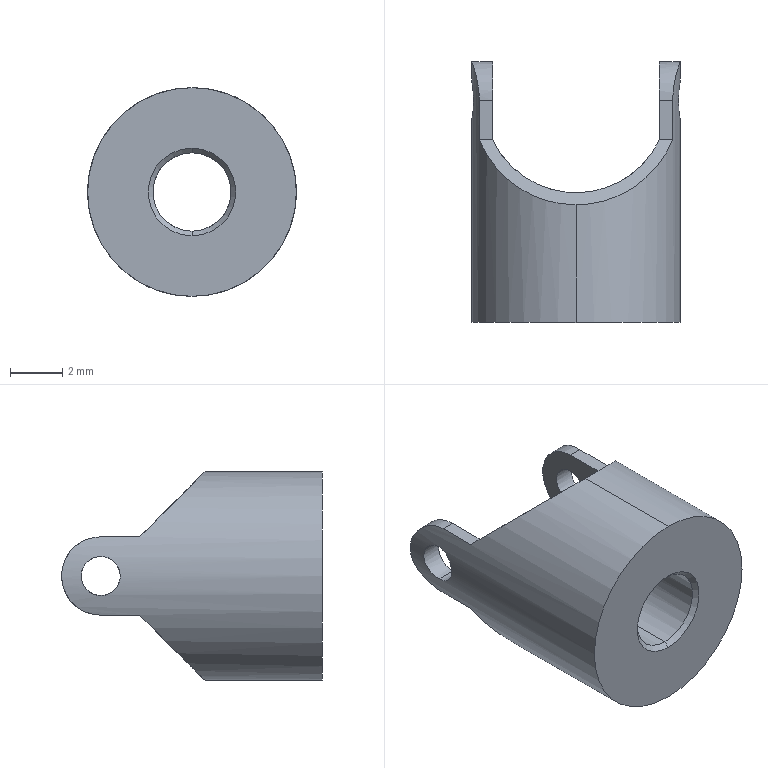Part | SolidWorks | features BaseBody 1, Scale 1 | 1 solid | 22 faces | box 8 x 10 x 8 mm | volume 253.333 mm3 | cylinder 11 | plane 9 | cone 2 | commonest cylinder face diameters 1.5 x4 3 x4 8 x2 7.068 x1
STEP:
#1=CARTESIAN_POINT('',(-3.2,8.5,-0.75));
#2=VERTEX_POINT('',#1);
#3=CARTESIAN_POINT('',(-3.2,8.5,0.75));
#4=VERTEX_POINT('',#3);
#5=CARTESIAN_POINT('',(-3.2,8.5,0.));
#6=DIRECTION('',(-1.,0.,0.));
#7=DIRECTION('',(0.,0.,-1.));
#8=AXIS2_PLACEMENT_3D('',#5,#6,#7);
#9=CIRCLE('',#8,0.75);
#10=EDGE_CURVE('',#2,#4,#9,.T.);
#11=ORIENTED_EDGE('',*,*,#10,.F.);
#12=CARTESIAN_POINT('',(-3.929,8.5,-0.75));
#13=VERTEX_POINT('',#12);
#14=CARTESIAN_POINT('',(4.,8.5,-0.75));
#15=DIRECTION('',(-1.,0.,0.));
#16=VECTOR('',#15,1000.);
#17=LINE('',#14,#16);
#18=EDGE_CURVE('',#2,#13,#17,.T.);
#19=ORIENTED_EDGE('',*,*,#18,.T.);
#20=CARTESIAN_POINT('',(-3.929,8.5,0.75));
#21=VERTEX_POINT('',#20);
#22=CARTESIAN_POINT('',(-3.929,8.5,0.75));
#23=CARTESIAN_POINT('',(-3.929,8.301,0.75));
#24=CARTESIAN_POINT('',(-3.946,8.107,0.668));
#25=CARTESIAN_POINT('',(-3.974,7.9,0.461));
#26=CARTESIAN_POINT('',(-3.983,7.845,0.3777));
#27=CARTESIAN_POINT('',(-3.996,7.77,0.1965));
#28=CARTESIAN_POINT('',(-4.,7.75,0.09865));
#29=CARTESIAN_POINT('',(-4.,7.75,-0.1985));
#30=CARTESIAN_POINT('',(-3.983,7.832,-0.3925));
#31=CARTESIAN_POINT('',(-3.946,8.108,-0.6688));
#32=CARTESIAN_POINT('',(-3.929,8.304,-0.75));
#33=CARTESIAN_POINT('',(-3.929,8.5,-0.75));
#34=B_SPLINE_CURVE_WITH_KNOTS('',3,(#22,#23,#24,#25,#26,#27,#28,#29,#30,#31,#32,#33),.UNSPECIFIED.,.F.,.F.,(4,2,2,2,2,4),(0.,0.0005912,0.0008868,0.001182,0.001774,0.002365),.UNSPECIFIED.);
#35=EDGE_CURVE('',#21,#13,#34,.T.);
#36=ORIENTED_EDGE('',*,*,#35,.F.);
#37=CARTESIAN_POINT('',(4.,8.5,0.75));
#38=DIRECTION('',(-1.,0.,0.));
#39=VECTOR('',#38,1000.);
#40=LINE('',#37,#39);
#41=EDGE_CURVE('',#4,#21,#40,.T.);
#42=ORIENTED_EDGE('',*,*,#41,.F.);
#43=EDGE_LOOP('',(#11,#19,#36,#42));
#44=FACE_OUTER_BOUND('',#43,.T.);
#45=CARTESIAN_POINT('',(4.,8.5,0.));
#46=DIRECTION('',(-1.,0.,0.));
#47=DIRECTION('',(0.,0.,1.));
#48=AXIS2_PLACEMENT_3D('',#45,#46,#47);
#49=CYLINDRICAL_SURFACE('',#48,0.75);
#50=ADVANCED_FACE('',(#44),#49,.F.);
#51=CARTESIAN_POINT('',(3.929,8.5,-0.75));
#52=VERTEX_POINT('',#51);
#53=CARTESIAN_POINT('',(3.929,8.5,0.75));
#54=VERTEX_POINT('',#53);
#55=CARTESIAN_POINT('',(3.929,8.5,-0.75));
#56=CARTESIAN_POINT('',(3.929,8.402,-0.75));
#57=CARTESIAN_POINT('',(3.933,8.303,-0.7304));
#58=CARTESIAN_POINT('',(3.946,8.122,-0.6552));
#59=CARTESIAN_POINT('',(3.955,8.039,-0.6001));
#60=CARTESIAN_POINT('',(3.974,7.9,-0.4606));
#61=CARTESIAN_POINT('',(3.983,7.845,-0.3781));
#62=CARTESIAN_POINT('',(3.996,7.769,-0.1962));
#63=CARTESIAN_POINT('',(4.,7.75,-0.09779));
#64=CARTESIAN_POINT('',(4.,7.75,0.1964));
#65=CARTESIAN_POINT('',(3.983,7.832,0.3921));
#66=CARTESIAN_POINT('',(3.955,8.039,0.5993));
#67=CARTESIAN_POINT('',(3.946,8.122,0.655));
#68=CARTESIAN_POINT('',(3.933,8.303,0.7304));
#69=CARTESIAN_POINT('',(3.929,8.401,0.75));
#70=CARTESIAN_POINT('',(3.929,8.5,0.75));
#71=B_SPLINE_CURVE_WITH_KNOTS('',3,(#55,#56,#57,#58,#59,#60,#61,#62,#63,#64,#65,#66,#67,#68,#69,#70),.UNSPECIFIED.,.F.,.F.,(4,2,2,2,2,2,2,4),(0.002365,0.00266,0.002956,0.003252,0.003547,0.004139,0.004434,0.00473),.UNSPECIFIED.);
#72=EDGE_CURVE('',#52,#54,#71,.T.);
#73=ORIENTED_EDGE('',*,*,#72,.F.);
#74=CARTESIAN_POINT('',(3.2,8.5,-0.75));
#75=VERTEX_POINT('',#74);
#76=CARTESIAN_POINT('',(4.,8.5,-0.75));
#77=DIRECTION('',(-1.,0.,0.));
#78=VECTOR('',#77,1000.);
#79=LINE('',#76,#78);
#80=EDGE_CURVE('',#52,#75,#79,.T.);
#81=ORIENTED_EDGE('',*,*,#80,.T.);
#82=CARTESIAN_POINT('',(3.2,8.5,0.75));
#83=VERTEX_POINT('',#82);
#84=CARTESIAN_POINT('',(3.2,8.5,0.));
#85=DIRECTION('',(1.,0.,0.));
#86=DIRECTION('',(0.,0.,1.));
#87=AXIS2_PLACEMENT_3D('',#84,#85,#86);
#88=CIRCLE('',#87,0.75);
#89=EDGE_CURVE('',#83,#75,#88,.T.);
#90=ORIENTED_EDGE('',*,*,#89,.F.);
#91=CARTESIAN_POINT('',(4.,8.5,0.75));
#92=DIRECTION('',(-1.,0.,0.));
#93=VECTOR('',#92,1000.);
#94=LINE('',#91,#93);
#95=EDGE_CURVE('',#54,#83,#94,.T.);
#96=ORIENTED_EDGE('',*,*,#95,.F.);
#97=EDGE_LOOP('',(#73,#81,#90,#96));
#98=FACE_OUTER_BOUND('',#97,.T.);
#99=CARTESIAN_POINT('',(4.,8.5,0.));
#100=DIRECTION('',(-1.,0.,0.));
#101=DIRECTION('',(0.,0.,1.));
#102=AXIS2_PLACEMENT_3D('',#99,#100,#101);
#103=CYLINDRICAL_SURFACE('',#102,0.75);
#104=ADVANCED_FACE('',(#98),#103,.F.);
#105=CARTESIAN_POINT('',(3.929,8.5,0.75));
#106=CARTESIAN_POINT('',(3.929,8.699,0.75));
#107=CARTESIAN_POINT('',(3.946,8.893,0.668));
#108=CARTESIAN_POINT('',(3.974,9.1,0.461));
#109=CARTESIAN_POINT('',(3.983,9.155,0.3777));
#110=CARTESIAN_POINT('',(3.996,9.23,0.1965));
#111=CARTESIAN_POINT('',(4.,9.25,0.09865));
#112=CARTESIAN_POINT('',(4.,9.25,-0.1985));
#113=CARTESIAN_POINT('',(3.983,9.168,-0.3925));
#114=CARTESIAN_POINT('',(3.946,8.892,-0.6688));
#115=CARTESIAN_POINT('',(3.929,8.696,-0.75));
#116=CARTESIAN_POINT('',(3.929,8.5,-0.75));
#117=B_SPLINE_CURVE_WITH_KNOTS('',3,(#105,#106,#107,#108,#109,#110,#111,#112,#113,#114,#115,#116),.UNSPECIFIED.,.F.,.F.,(4,2,2,2,2,4),(0.,0.0005912,0.0008868,0.001182,0.001774,0.002365),.UNSPECIFIED.);
#118=EDGE_CURVE('',#54,#52,#117,.T.);
#119=ORIENTED_EDGE('',*,*,#118,.T.);
#120=ORIENTED_EDGE('',*,*,#72,.T.);
#121=EDGE_LOOP('',(#119,#120));
#122=FACE_BOUND('',#121,.T.);
#123=CARTESIAN_POINT('',(0.,4.5,4.));
#124=VERTEX_POINT('',#123);
#125=CARTESIAN_POINT('',(3.708,7.,1.5));
#126=VERTEX_POINT('',#125);
#127=CARTESIAN_POINT('',(0.,4.5,4.));
#128=CARTESIAN_POINT('',(1.682,4.5,4.));
#129=CARTESIAN_POINT('',(3.077,5.44,3.06));
#130=CARTESIAN_POINT('',(3.708,7.,1.5));
#131=(BOUNDED_CURVE()B_SPLINE_CURVE(3,(#127,#128,#129,#130),.UNSPECIFIED.,.F.,.F.)B_SPLINE_CURVE_WITH_KNOTS((4,4),(0.,1.186),.UNSPECIFIED.)CURVE()GEOMETRIC_REPRESENTATION_ITEM()RATIONAL_B_SPLINE_CURVE((1.,0.8861,0.8861,1.))REPRESENTATION_ITEM(''));
#132=EDGE_CURVE('',#124,#126,#131,.T.);
#133=ORIENTED_EDGE('',*,*,#132,.F.);
#134=CARTESIAN_POINT('',(0.,0.,4.));
#135=VERTEX_POINT('',#134);
#136=CARTESIAN_POINT('',(0.,10.,4.));
#137=DIRECTION('',(0.,-1.,0.));
#138=VECTOR('',#137,1000.);
#139=LINE('',#136,#138);
#140=EDGE_CURVE('',#124,#135,#139,.T.);
#141=ORIENTED_EDGE('',*,*,#140,.T.);
#142=CARTESIAN_POINT('',(0.,0.,-4.));
#143=VERTEX_POINT('',#142);
#144=CARTESIAN_POINT('',(0.,0.,0.));
#145=DIRECTION('',(0.,1.,0.));
#146=DIRECTION('',(1.,0.,0.));
#147=AXIS2_PLACEMENT_3D('',#144,#145,#146);
#148=CIRCLE('',#147,4.);
#149=EDGE_CURVE('',#135,#143,#148,.T.);
#150=ORIENTED_EDGE('',*,*,#149,.T.);
#151=CARTESIAN_POINT('',(0.,4.5,-4.));
#152=VERTEX_POINT('',#151);
#153=CARTESIAN_POINT('',(0.,10.,-4.));
#154=DIRECTION('',(0.,-1.,0.));
#155=VECTOR('',#154,1000.);
#156=LINE('',#153,#155);
#157=EDGE_CURVE('',#152,#143,#156,.T.);
#158=ORIENTED_EDGE('',*,*,#157,.F.);
#159=CARTESIAN_POINT('',(3.708,7.,-1.5));
#160=VERTEX_POINT('',#159);
#161=CARTESIAN_POINT('',(3.708,7.,-1.5));
#162=CARTESIAN_POINT('',(3.077,5.44,-3.06));
#163=CARTESIAN_POINT('',(1.682,4.5,-4.));
#164=CARTESIAN_POINT('',(0.,4.5,-4.));
#165=(BOUNDED_CURVE()B_SPLINE_CURVE(3,(#161,#162,#163,#164),.UNSPECIFIED.,.F.,.F.)B_SPLINE_CURVE_WITH_KNOTS((4,4),(5.097,6.283),.UNSPECIFIED.)CURVE()GEOMETRIC_REPRESENTATION_ITEM()RATIONAL_B_SPLINE_CURVE((1.,0.8861,0.8861,1.))REPRESENTATION_ITEM(''));
#166=EDGE_CURVE('',#160,#152,#165,.T.);
#167=ORIENTED_EDGE('',*,*,#166,.F.);
#168=CARTESIAN_POINT('',(3.708,8.5,-1.5));
#169=VERTEX_POINT('',#168);
#170=CARTESIAN_POINT('',(3.708,10.,-1.5));
#171=DIRECTION('',(0.,-1.,0.));
#172=VECTOR('',#171,1000.);
#173=LINE('',#170,#172);
#174=EDGE_CURVE('',#169,#160,#173,.T.);
#175=ORIENTED_EDGE('',*,*,#174,.F.);
#176=CARTESIAN_POINT('',(3.708,8.5,1.5));
#177=VERTEX_POINT('',#176);
#178=CARTESIAN_POINT('',(3.708,8.5,1.5));
#179=CARTESIAN_POINT('',(3.708,8.6,1.5));
#180=CARTESIAN_POINT('',(3.712,8.698,1.49));
#181=CARTESIAN_POINT('',(3.727,8.891,1.451));
#182=CARTESIAN_POINT('',(3.739,8.987,1.422));
#183=CARTESIAN_POINT('',(3.781,9.258,1.309));
#184=CARTESIAN_POINT('',(3.819,9.423,1.198));
#185=CARTESIAN_POINT('',(3.894,9.697,0.924));
#186=CARTESIAN_POINT('',(3.932,9.809,0.7582));
#187=CARTESIAN_POINT('',(3.971,9.922,0.488));
#188=CARTESIAN_POINT('',(3.982,9.951,0.3926));
#189=CARTESIAN_POINT('',(3.996,9.99,0.1986));
#190=CARTESIAN_POINT('',(4.,10.,0.1006));
#191=CARTESIAN_POINT('',(4.,10.,-0.09712));
#192=CARTESIAN_POINT('',(3.996,9.99,-0.1975));
#193=CARTESIAN_POINT('',(3.982,9.952,-0.3907));
#194=CARTESIAN_POINT('',(3.972,9.923,-0.4847));
#195=CARTESIAN_POINT('',(3.932,9.809,-0.759));
#196=CARTESIAN_POINT('',(3.895,9.698,-0.9229));
#197=CARTESIAN_POINT('',(3.838,9.492,-1.129));
#198=CARTESIAN_POINT('',(3.819,9.417,-1.191));
#199=CARTESIAN_POINT('',(3.783,9.256,-1.299));
#200=CARTESIAN_POINT('',(3.767,9.168,-1.347));
#201=CARTESIAN_POINT('',(3.725,8.898,-1.459));
#202=CARTESIAN_POINT('',(3.708,8.7,-1.5));
#203=CARTESIAN_POINT('',(3.708,8.5,-1.5));
#204=B_SPLINE_CURVE_WITH_KNOTS('',3,(#178,#179,#180,#181,#182,#183,#184,#185,#186,#187,#188,#189,#190,#191,#192,#193,#194,#195,#196,#197,#198,#199,#200,#201,#202,#203),.UNSPECIFIED.,.F.,.F.,(4,2,2,2,2,2,2,2,2,2,2,2,4),(0.,0.0002957,0.0005914,0.001183,0.001774,0.00207,0.002366,0.002661,0.002957,0.003548,0.003844,0.00414,0.004731),.UNSPECIFIED.);
#205=EDGE_CURVE('',#177,#169,#204,.T.);
#206=ORIENTED_EDGE('',*,*,#205,.F.);
#207=CARTESIAN_POINT('',(3.708,10.,1.5));
#208=DIRECTION('',(0.,1.,0.));
#209=VECTOR('',#208,1000.);
#210=LINE('',#207,#209);
#211=EDGE_CURVE('',#126,#177,#210,.T.);
#212=ORIENTED_EDGE('',*,*,#211,.F.);
#213=EDGE_LOOP('',(#133,#141,#150,#158,#167,#175,#206,#212));
#214=FACE_OUTER_BOUND('',#213,.T.);
#215=CARTESIAN_POINT('',(0.,10.,0.));
#216=DIRECTION('',(0.,-1.,0.));
#217=DIRECTION('',(0.,0.,-1.));
#218=AXIS2_PLACEMENT_3D('',#215,#216,#217);
#219=CYLINDRICAL_SURFACE('',#218,4.);
#220=ADVANCED_FACE('',(#122,#214),#219,.T.);
#221=CARTESIAN_POINT('',(0.,4.966,1.5));
#222=VERTEX_POINT('',#221);
#223=CARTESIAN_POINT('',(0.,4.966,-1.5));
#224=VERTEX_POINT('',#223);
#225=CARTESIAN_POINT('',(0.,4.966,1.5));
#226=CARTESIAN_POINT('',(-0.09881,4.966,1.5));
#227=CARTESIAN_POINT('',(-0.1992,4.97,1.49));
#228=CARTESIAN_POINT('',(-0.3935,4.987,1.451));
#229=CARTESIAN_POINT('',(-0.4874,4.998,1.422));
#230=CARTESIAN_POINT('',(-0.76,5.044,1.308));
#231=CARTESIAN_POINT('',(-0.9239,5.086,1.198));
#232=CARTESIAN_POINT('',(-1.13,5.151,0.9907));
#233=CARTESIAN_POINT('',(-1.192,5.172,0.916));
#234=CARTESIAN_POINT('',(-1.3,5.213,0.7551));
#235=CARTESIAN_POINT('',(-1.347,5.232,0.6678));
#236=CARTESIAN_POINT('',(-1.422,5.264,0.4871));
#237=CARTESIAN_POINT('',(-1.451,5.277,0.3937));
#238=CARTESIAN_POINT('',(-1.49,5.295,0.2));
#239=CARTESIAN_POINT('',(-1.5,5.3,0.09937));
#240=CARTESIAN_POINT('',(-1.5,5.3,-0.1973));
#241=CARTESIAN_POINT('',(-1.46,5.28,-0.3966));
#242=CARTESIAN_POINT('',(-1.347,5.232,-0.6676));
#243=CARTESIAN_POINT('',(-1.3,5.213,-0.755));
#244=CARTESIAN_POINT('',(-1.192,5.172,-0.9164));
#245=CARTESIAN_POINT('',(-1.13,5.151,-0.9911));
#246=CARTESIAN_POINT('',(-0.9236,5.086,-1.198));
#247=CARTESIAN_POINT('',(-0.7612,5.044,-1.308));
#248=CARTESIAN_POINT('',(-0.3959,4.983,-1.46));
#249=CARTESIAN_POINT('',(-0.2006,4.966,-1.5));
#250=CARTESIAN_POINT('',(0.,4.966,-1.5));
#251=B_SPLINE_CURVE_WITH_KNOTS('',3,(#225,#226,#227,#228,#229,#230,#231,#232,#233,#234,#235,#236,#237,#238,#239,#240,#241,#242,#243,#244,#245,#246,#247,#248,#249,#250),.UNSPECIFIED.,.F.,.F.,(4,2,2,2,2,2,2,2,2,2,2,2,4),(0.004747,0.005043,0.005339,0.005932,0.006229,0.006525,0.006822,0.007118,0.007711,0.008007,0.008304,0.008896,0.009489),.UNSPECIFIED.);
#252=EDGE_CURVE('',#222,#224,#251,.T.);
#253=ORIENTED_EDGE('',*,*,#252,.F.);
#254=CARTESIAN_POINT('',(0.,0.18,1.5));
#255=VERTEX_POINT('',#254);
#256=CARTESIAN_POINT('',(0.,15.1,1.5));
#257=DIRECTION('',(0.,-1.,0.));
#258=VECTOR('',#257,1000.);
#259=LINE('',#256,#258);
#260=EDGE_CURVE('',#222,#255,#259,.T.);
#261=ORIENTED_EDGE('',*,*,#260,.T.);
#262=CARTESIAN_POINT('',(0.,0.18,-1.5));
#263=VERTEX_POINT('',#262);
#264=CARTESIAN_POINT('',(0.,0.18,0.));
#265=DIRECTION('',(0.,-1.,0.));
#266=DIRECTION('',(0.,0.,1.));
#267=AXIS2_PLACEMENT_3D('',#264,#265,#266);
#268=CIRCLE('',#267,1.5);
#269=EDGE_CURVE('',#255,#263,#268,.T.);
#270=ORIENTED_EDGE('',*,*,#269,.T.);
#271=CARTESIAN_POINT('',(0.,15.1,-1.5));
#272=DIRECTION('',(0.,-1.,0.));
#273=VECTOR('',#272,1000.);
#274=LINE('',#271,#273);
#275=EDGE_CURVE('',#224,#263,#274,.T.);
#276=ORIENTED_EDGE('',*,*,#275,.F.);
#277=EDGE_LOOP('',(#253,#261,#270,#276));
#278=FACE_OUTER_BOUND('',#277,.T.);
#279=CARTESIAN_POINT('',(0.,15.1,0.));
#280=DIRECTION('',(0.,-1.,0.));
#281=DIRECTION('',(0.,0.,-1.));
#282=AXIS2_PLACEMENT_3D('',#279,#280,#281);
#283=CYLINDRICAL_SURFACE('',#282,1.5);
#284=ADVANCED_FACE('',(#278),#283,.F.);
#285=ORIENTED_EDGE('',*,*,#269,.F.);
#286=CARTESIAN_POINT('',(0.,0.,1.68));
#287=VERTEX_POINT('',#286);
#288=CARTESIAN_POINT('',(0.,0.,1.68));
#289=DIRECTION('',(0.,-0.7071,0.7071));
#290=VECTOR('',#289,1000.);
#291=LINE('',#288,#290);
#292=EDGE_CURVE('',#255,#287,#291,.T.);
#293=ORIENTED_EDGE('',*,*,#292,.T.);
#294=CARTESIAN_POINT('',(0.,0.,-1.68));
#295=VERTEX_POINT('',#294);
#296=CARTESIAN_POINT('',(0.,0.,0.));
#297=DIRECTION('',(0.,1.,0.));
#298=DIRECTION('',(0.,0.,1.));
#299=AXIS2_PLACEMENT_3D('',#296,#297,#298);
#300=CIRCLE('',#299,1.68);
#301=EDGE_CURVE('',#295,#287,#300,.T.);
#302=ORIENTED_EDGE('',*,*,#301,.F.);
#303=CARTESIAN_POINT('',(0.,0.,-1.68));
#304=DIRECTION('',(0.,-0.7071,-0.7071));
#305=VECTOR('',#304,1000.);
#306=LINE('',#303,#305);
#307=EDGE_CURVE('',#263,#295,#306,.T.);
#308=ORIENTED_EDGE('',*,*,#307,.F.);
#309=EDGE_LOOP('',(#285,#293,#302,#308));
#310=FACE_OUTER_BOUND('',#309,.T.);
#311=CARTESIAN_POINT('',(0.,0.,0.));
#312=DIRECTION('',(0.,-1.,0.));
#313=DIRECTION('',(0.,0.,-1.));
#314=AXIS2_PLACEMENT_3D('',#311,#312,#313);
#315=CONICAL_SURFACE('',#314,1.68,0.7854);
#316=ADVANCED_FACE('',(#310),#315,.F.);
#317=ORIENTED_EDGE('',*,*,#292,.F.);
#318=CARTESIAN_POINT('',(0.,0.18,0.));
#319=DIRECTION('',(0.,-1.,0.));
#320=DIRECTION('',(0.,0.,1.));
#321=AXIS2_PLACEMENT_3D('',#318,#319,#320);
#322=CIRCLE('',#321,1.5);
#323=EDGE_CURVE('',#263,#255,#322,.T.);
#324=ORIENTED_EDGE('',*,*,#323,.F.);
#325=ORIENTED_EDGE('',*,*,#307,.T.);
#326=CARTESIAN_POINT('',(0.,0.,0.));
#327=DIRECTION('',(0.,1.,0.));
#328=DIRECTION('',(0.,0.,1.));
#329=AXIS2_PLACEMENT_3D('',#326,#327,#328);
#330=CIRCLE('',#329,1.68);
#331=EDGE_CURVE('',#287,#295,#330,.T.);
#332=ORIENTED_EDGE('',*,*,#331,.F.);
#333=EDGE_LOOP('',(#317,#324,#325,#332));
#334=FACE_OUTER_BOUND('',#333,.T.);
#335=CARTESIAN_POINT('',(0.,0.,0.));
#336=DIRECTION('',(0.,-1.,0.));
#337=DIRECTION('',(0.,0.,-1.));
#338=AXIS2_PLACEMENT_3D('',#335,#336,#337);
#339=CONICAL_SURFACE('',#338,1.68,0.7854);
#340=ADVANCED_FACE('',(#334),#339,.F.);
#341=ORIENTED_EDGE('',*,*,#260,.F.);
#342=CARTESIAN_POINT('',(0.,4.966,-1.5));
#343=CARTESIAN_POINT('',(0.1004,4.966,-1.5));
#344=CARTESIAN_POINT('',(0.1989,4.97,-1.49));
#345=CARTESIAN_POINT('',(0.3923,4.986,-1.451));
#346=CARTESIAN_POINT('',(0.4882,4.999,-1.422));
#347=CARTESIAN_POINT('',(0.7601,5.044,-1.308));
#348=CARTESIAN_POINT('',(0.9249,5.086,-1.197));
#349=CARTESIAN_POINT('',(1.198,5.172,-0.9231));
#350=CARTESIAN_POINT('',(1.309,5.216,-0.7581));
#351=CARTESIAN_POINT('',(1.422,5.264,-0.4882));
#352=CARTESIAN_POINT('',(1.451,5.277,-0.3925));
#353=CARTESIAN_POINT('',(1.49,5.295,-0.1983));
#354=CARTESIAN_POINT('',(1.5,5.3,-0.1002));
#355=CARTESIAN_POINT('',(1.5,5.3,0.0982));
#356=CARTESIAN_POINT('',(1.49,5.295,0.1989));
#357=CARTESIAN_POINT('',(1.451,5.277,0.3924));
#358=CARTESIAN_POINT('',(1.422,5.264,0.4869));
#359=CARTESIAN_POINT('',(1.346,5.232,0.6693));
#360=CARTESIAN_POINT('',(1.3,5.213,0.755));
#361=CARTESIAN_POINT('',(1.192,5.172,0.9164));
#362=CARTESIAN_POINT('',(1.129,5.15,0.9925));
#363=CARTESIAN_POINT('',(0.9233,5.086,1.198));
#364=CARTESIAN_POINT('',(0.758,5.043,1.309));
#365=CARTESIAN_POINT('',(0.3975,4.984,1.46));
#366=CARTESIAN_POINT('',(0.1978,4.966,1.5));
#367=CARTESIAN_POINT('',(0.,4.966,1.5));
#368=B_SPLINE_CURVE_WITH_KNOTS('',3,(#342,#343,#344,#345,#346,#347,#348,#349,#350,#351,#352,#353,#354,#355,#356,#357,#358,#359,#360,#361,#362,#363,#364,#365,#366,#367),.UNSPECIFIED.,.F.,.F.,(4,2,2,2,2,2,2,2,2,2,2,2,4),(0.,0.0002967,0.0005933,0.001187,0.00178,0.002077,0.002373,0.00267,0.002967,0.003263,0.00356,0.004153,0.004747),.UNSPECIFIED.);
#369=EDGE_CURVE('',#224,#222,#368,.T.);
#370=ORIENTED_EDGE('',*,*,#369,.F.);
#371=ORIENTED_EDGE('',*,*,#275,.T.);
#372=ORIENTED_EDGE('',*,*,#323,.T.);
#373=EDGE_LOOP('',(#341,#370,#371,#372));
#374=FACE_OUTER_BOUND('',#373,.T.);
#375=CARTESIAN_POINT('',(0.,15.1,0.));
#376=DIRECTION('',(0.,-1.,0.));
#377=DIRECTION('',(0.,0.,-1.));
#378=AXIS2_PLACEMENT_3D('',#375,#376,#377);
#379=CYLINDRICAL_SURFACE('',#378,1.5);
#380=ADVANCED_FACE('',(#374),#379,.F.);
#381=ORIENTED_EDGE('',*,*,#89,.T.);
#382=CARTESIAN_POINT('',(3.2,8.5,0.));
#383=DIRECTION('',(1.,0.,0.));
#384=DIRECTION('',(0.,0.,1.));
#385=AXIS2_PLACEMENT_3D('',#382,#383,#384);
#386=CIRCLE('',#385,0.75);
#387=EDGE_CURVE('',#75,#83,#386,.T.);
#388=ORIENTED_EDGE('',*,*,#387,.T.);
#389=EDGE_LOOP('',(#381,#388));
#390=FACE_BOUND('',#389,.T.);
#391=CARTESIAN_POINT('',(3.2,8.5,-1.5));
#392=VERTEX_POINT('',#391);
#393=CARTESIAN_POINT('',(3.2,8.5,1.5));
#394=VERTEX_POINT('',#393);
#395=CARTESIAN_POINT('',(3.2,8.5,0.));
#396=DIRECTION('',(1.,0.,0.));
#397=DIRECTION('',(0.,0.,1.));
#398=AXIS2_PLACEMENT_3D('',#395,#396,#397);
#399=CIRCLE('',#398,1.5);
#400=EDGE_CURVE('',#392,#394,#399,.T.);
#401=ORIENTED_EDGE('',*,*,#400,.F.);
#402=CARTESIAN_POINT('',(3.2,7.,-1.5));
#403=VERTEX_POINT('',#402);
#404=CARTESIAN_POINT('',(3.2,8.5,-1.5));
#405=DIRECTION('',(0.,1.,0.));
#406=VECTOR('',#405,1000.);
#407=LINE('',#404,#406);
#408=EDGE_CURVE('',#403,#392,#407,.T.);
#409=ORIENTED_EDGE('',*,*,#408,.F.);
#410=CARTESIAN_POINT('',(3.2,7.,1.5));
#411=VERTEX_POINT('',#410);
#412=CARTESIAN_POINT('',(3.2,7.,4.));
#413=DIRECTION('',(0.,0.,-1.));
#414=VECTOR('',#413,1000.);
#415=LINE('',#412,#414);
#416=EDGE_CURVE('',#411,#403,#415,.T.);
#417=ORIENTED_EDGE('',*,*,#416,.F.);
#418=CARTESIAN_POINT('',(3.2,8.5,1.5));
#419=DIRECTION('',(0.,-1.,0.));
#420=VECTOR('',#419,1000.);
#421=LINE('',#418,#420);
#422=EDGE_CURVE('',#394,#411,#421,.T.);
#423=ORIENTED_EDGE('',*,*,#422,.F.);
#424=EDGE_LOOP('',(#401,#409,#417,#423));
#425=FACE_OUTER_BOUND('',#424,.T.);
#426=CARTESIAN_POINT('',(3.2,10.,4.));
#427=DIRECTION('',(-1.,0.,0.));
#428=DIRECTION('',(0.,0.,1.));
#429=AXIS2_PLACEMENT_3D('',#426,#427,#428);
#430=PLANE('',#429);
#431=ADVANCED_FACE('',(#390,#425),#430,.T.);
#432=CARTESIAN_POINT('',(-3.2,8.5,0.));
#433=DIRECTION('',(-1.,0.,0.));
#434=DIRECTION('',(0.,0.,-1.));
#435=AXIS2_PLACEMENT_3D('',#432,#433,#434);
#436=CIRCLE('',#435,0.75);
#437=EDGE_CURVE('',#4,#2,#436,.T.);
#438=ORIENTED_EDGE('',*,*,#437,.T.);
#439=ORIENTED_EDGE('',*,*,#10,.T.);
#440=EDGE_LOOP('',(#438,#439));
#441=FACE_BOUND('',#440,.T.);
#442=CARTESIAN_POINT('',(-3.2,7.,1.5));
#443=VERTEX_POINT('',#442);
#444=CARTESIAN_POINT('',(-3.2,7.,-1.5));
#445=VERTEX_POINT('',#444);
#446=CARTESIAN_POINT('',(-3.2,7.,4.));
#447=DIRECTION('',(0.,0.,-1.));
#448=VECTOR('',#447,1000.);
#449=LINE('',#446,#448);
#450=EDGE_CURVE('',#443,#445,#449,.T.);
#451=ORIENTED_EDGE('',*,*,#450,.T.);
#452=CARTESIAN_POINT('',(-3.2,8.5,-1.5));
#453=VERTEX_POINT('',#452);
#454=CARTESIAN_POINT('',(-3.2,8.5,-1.5));
#455=DIRECTION('',(0.,-1.,0.));
#456=VECTOR('',#455,1000.);
#457=LINE('',#454,#456);
#458=EDGE_CURVE('',#453,#445,#457,.T.);
#459=ORIENTED_EDGE('',*,*,#458,.F.);
#460=CARTESIAN_POINT('',(-3.2,8.5,1.5));
#461=VERTEX_POINT('',#460);
#462=CARTESIAN_POINT('',(-3.2,8.5,0.));
#463=DIRECTION('',(-1.,0.,0.));
#464=DIRECTION('',(0.,0.,-1.));
#465=AXIS2_PLACEMENT_3D('',#462,#463,#464);
#466=CIRCLE('',#465,1.5);
#467=EDGE_CURVE('',#461,#453,#466,.T.);
#468=ORIENTED_EDGE('',*,*,#467,.F.);
#469=CARTESIAN_POINT('',(-3.2,8.5,1.5));
#470=DIRECTION('',(0.,1.,0.));
#471=VECTOR('',#470,1000.);
#472=LINE('',#469,#471);
#473=EDGE_CURVE('',#443,#461,#472,.T.);
#474=ORIENTED_EDGE('',*,*,#473,.F.);
#475=EDGE_LOOP('',(#451,#459,#468,#474));
#476=FACE_OUTER_BOUND('',#475,.T.);
#477=CARTESIAN_POINT('',(-3.2,10.,4.));
#478=DIRECTION('',(1.,0.,0.));
#479=DIRECTION('',(0.,1.,0.));
#480=AXIS2_PLACEMENT_3D('',#477,#478,#479);
#481=PLANE('',#480);
#482=ADVANCED_FACE('',(#441,#476),#481,.T.);
#483=CARTESIAN_POINT('',(-3.708,7.,-1.5));
#484=VERTEX_POINT('',#483);
#485=CARTESIAN_POINT('',(4.,7.,-1.5));
#486=DIRECTION('',(-1.,0.,0.));
#487=VECTOR('',#486,1000.);
#488=LINE('',#485,#487);
#489=EDGE_CURVE('',#445,#484,#488,.T.);
#490=ORIENTED_EDGE('',*,*,#489,.F.);
#491=CARTESIAN_POINT('',(-3.2,7.,-1.5));
#492=CARTESIAN_POINT('',(-1.731,3.866,-4.634));
#493=CARTESIAN_POINT('',(1.731,3.866,-4.634));
#494=CARTESIAN_POINT('',(3.2,7.,-1.5));
#495=(BOUNDED_CURVE()B_SPLINE_CURVE(3,(#491,#492,#493,#494),.UNSPECIFIED.,.F.,.F.)B_SPLINE_CURVE_WITH_KNOTS((4,4),(5.151,7.416),.UNSPECIFIED.)CURVE()GEOMETRIC_REPRESENTATION_ITEM()RATIONAL_B_SPLINE_CURVE((1.,0.6163,0.6163,1.))REPRESENTATION_ITEM(''));
#496=EDGE_CURVE('',#445,#403,#495,.T.);
#497=ORIENTED_EDGE('',*,*,#496,.T.);
#498=CARTESIAN_POINT('',(4.,7.,-1.5));
#499=DIRECTION('',(-1.,0.,0.));
#500=VECTOR('',#499,1000.);
#501=LINE('',#498,#500);
#502=EDGE_CURVE('',#160,#403,#501,.T.);
#503=ORIENTED_EDGE('',*,*,#502,.F.);
#504=ORIENTED_EDGE('',*,*,#166,.T.);
#505=CARTESIAN_POINT('',(0.,4.5,-4.));
#506=CARTESIAN_POINT('',(-1.682,4.5,-4.));
#507=CARTESIAN_POINT('',(-3.077,5.44,-3.06));
#508=CARTESIAN_POINT('',(-3.708,7.,-1.5));
#509=(BOUNDED_CURVE()B_SPLINE_CURVE(3,(#505,#506,#507,#508),.UNSPECIFIED.,.F.,.F.)B_SPLINE_CURVE_WITH_KNOTS((4,4),(0.,1.186),.UNSPECIFIED.)CURVE()GEOMETRIC_REPRESENTATION_ITEM()RATIONAL_B_SPLINE_CURVE((1.,0.8861,0.8861,1.))REPRESENTATION_ITEM(''));
#510=EDGE_CURVE('',#152,#484,#509,.T.);
#511=ORIENTED_EDGE('',*,*,#510,.T.);
#512=EDGE_LOOP('',(#490,#497,#503,#504,#511));
#513=FACE_OUTER_BOUND('',#512,.T.);
#514=CARTESIAN_POINT('',(4.,7.,-1.5));
#515=DIRECTION('',(0.,0.7071,-0.7071));
#516=DIRECTION('',(-1.,0.,0.));
#517=AXIS2_PLACEMENT_3D('',#514,#515,#516);
#518=PLANE('',#517);
#519=ADVANCED_FACE('',(#513),#518,.T.);
#520=CARTESIAN_POINT('',(4.,7.,1.5));
#521=DIRECTION('',(-1.,0.,0.));
#522=VECTOR('',#521,1000.);
#523=LINE('',#520,#522);
#524=EDGE_CURVE('',#126,#411,#523,.T.);
#525=ORIENTED_EDGE('',*,*,#524,.T.);
#526=CARTESIAN_POINT('',(3.2,7.,1.5));
#527=CARTESIAN_POINT('',(1.731,3.866,4.634));
#528=CARTESIAN_POINT('',(-1.731,3.866,4.634));
#529=CARTESIAN_POINT('',(-3.2,7.,1.5));
#530=(BOUNDED_CURVE()B_SPLINE_CURVE(3,(#526,#527,#528,#529),.UNSPECIFIED.,.F.,.F.)B_SPLINE_CURVE_WITH_KNOTS((4,4),(2.009,4.274),.UNSPECIFIED.)CURVE()GEOMETRIC_REPRESENTATION_ITEM()RATIONAL_B_SPLINE_CURVE((1.,0.6163,0.6163,1.))REPRESENTATION_ITEM(''));
#531=EDGE_CURVE('',#411,#443,#530,.T.);
#532=ORIENTED_EDGE('',*,*,#531,.T.);
#533=CARTESIAN_POINT('',(-3.708,7.,1.5));
#534=VERTEX_POINT('',#533);
#535=CARTESIAN_POINT('',(4.,7.,1.5));
#536=DIRECTION('',(-1.,0.,0.));
#537=VECTOR('',#536,1000.);
#538=LINE('',#535,#537);
#539=EDGE_CURVE('',#443,#534,#538,.T.);
#540=ORIENTED_EDGE('',*,*,#539,.T.);
#541=CARTESIAN_POINT('',(-3.708,7.,1.5));
#542=CARTESIAN_POINT('',(-3.077,5.44,3.06));
#543=CARTESIAN_POINT('',(-1.682,4.5,4.));
#544=CARTESIAN_POINT('',(0.,4.5,4.));
#545=(BOUNDED_CURVE()B_SPLINE_CURVE(3,(#541,#542,#543,#544),.UNSPECIFIED.,.F.,.F.)B_SPLINE_CURVE_WITH_KNOTS((4,4),(5.097,6.283),.UNSPECIFIED.)CURVE()GEOMETRIC_REPRESENTATION_ITEM()RATIONAL_B_SPLINE_CURVE((1.,0.8861,0.8861,1.))REPRESENTATION_ITEM(''));
#546=EDGE_CURVE('',#534,#124,#545,.T.);
#547=ORIENTED_EDGE('',*,*,#546,.T.);
#548=ORIENTED_EDGE('',*,*,#132,.T.);
#549=EDGE_LOOP('',(#525,#532,#540,#547,#548));
#550=FACE_OUTER_BOUND('',#549,.T.);
#551=CARTESIAN_POINT('',(4.,7.,1.5));
#552=DIRECTION('',(0.,0.7071,0.7071));
#553=DIRECTION('',(1.,0.,0.));
#554=AXIS2_PLACEMENT_3D('',#551,#552,#553);
#555=PLANE('',#554);
#556=ADVANCED_FACE('',(#550),#555,.T.);
#557=CARTESIAN_POINT('',(0.,0.,0.));
#558=DIRECTION('',(0.,1.,0.));
#559=DIRECTION('',(1.,0.,0.));
#560=AXIS2_PLACEMENT_3D('',#557,#558,#559);
#561=CIRCLE('',#560,4.);
#562=EDGE_CURVE('',#143,#135,#561,.T.);
#563=ORIENTED_EDGE('',*,*,#562,.F.);
#564=ORIENTED_EDGE('',*,*,#149,.F.);
#565=EDGE_LOOP('',(#563,#564));
#566=FACE_OUTER_BOUND('',#565,.T.);
#567=ORIENTED_EDGE('',*,*,#301,.T.);
#568=ORIENTED_EDGE('',*,*,#331,.T.);
#569=EDGE_LOOP('',(#567,#568));
#570=FACE_BOUND('',#569,.T.);
#571=CARTESIAN_POINT('',(0.,0.,0.));
#572=DIRECTION('',(0.,1.,0.));
#573=DIRECTION('',(1.,0.,0.));
#574=AXIS2_PLACEMENT_3D('',#571,#572,#573);
#575=PLANE('',#574);
#576=ADVANCED_FACE('',(#566,#570),#575,.F.);
#577=ORIENTED_EDGE('',*,*,#140,.F.);
#578=ORIENTED_EDGE('',*,*,#546,.F.);
#579=CARTESIAN_POINT('',(-3.708,8.5,1.5));
#580=VERTEX_POINT('',#579);
#581=CARTESIAN_POINT('',(-3.708,10.,1.5));
#582=DIRECTION('',(0.,-1.,0.));
#583=VECTOR('',#582,1000.);
#584=LINE('',#581,#583);
#585=EDGE_CURVE('',#580,#534,#584,.T.);
#586=ORIENTED_EDGE('',*,*,#585,.F.);
#587=CARTESIAN_POINT('',(-3.708,8.5,-1.5));
#588=VERTEX_POINT('',#587);
#589=CARTESIAN_POINT('',(-3.708,8.5,-1.5));
#590=CARTESIAN_POINT('',(-3.708,8.6,-1.5));
#591=CARTESIAN_POINT('',(-3.712,8.698,-1.49));
#592=CARTESIAN_POINT('',(-3.727,8.891,-1.451));
#593=CARTESIAN_POINT('',(-3.739,8.987,-1.422));
#594=CARTESIAN_POINT('',(-3.781,9.258,-1.309));
#595=CARTESIAN_POINT('',(-3.819,9.423,-1.198));
#596=CARTESIAN_POINT('',(-3.894,9.697,-0.924));
#597=CARTESIAN_POINT('',(-3.932,9.809,-0.7582));
#598=CARTESIAN_POINT('',(-3.971,9.922,-0.488));
#599=CARTESIAN_POINT('',(-3.982,9.951,-0.3926));
#600=CARTESIAN_POINT('',(-3.996,9.99,-0.1986));
#601=CARTESIAN_POINT('',(-4.,10.,-0.1006));
#602=CARTESIAN_POINT('',(-4.,10.,0.09712));
#603=CARTESIAN_POINT('',(-3.996,9.99,0.1975));
#604=CARTESIAN_POINT('',(-3.982,9.952,0.3907));
#605=CARTESIAN_POINT('',(-3.972,9.923,0.4847));
#606=CARTESIAN_POINT('',(-3.932,9.809,0.759));
#607=CARTESIAN_POINT('',(-3.895,9.698,0.9229));
#608=CARTESIAN_POINT('',(-3.838,9.492,1.129));
#609=CARTESIAN_POINT('',(-3.819,9.417,1.191));
#610=CARTESIAN_POINT('',(-3.783,9.256,1.299));
#611=CARTESIAN_POINT('',(-3.767,9.168,1.347));
#612=CARTESIAN_POINT('',(-3.725,8.898,1.459));
#613=CARTESIAN_POINT('',(-3.708,8.7,1.5));
#614=CARTESIAN_POINT('',(-3.708,8.5,1.5));
#615=B_SPLINE_CURVE_WITH_KNOTS('',3,(#589,#590,#591,#592,#593,#594,#595,#596,#597,#598,#599,#600,#601,#602,#603,#604,#605,#606,#607,#608,#609,#610,#611,#612,#613,#614),.UNSPECIFIED.,.F.,.F.,(4,2,2,2,2,2,2,2,2,2,2,2,4),(0.,0.0002957,0.0005914,0.001183,0.001774,0.00207,0.002366,0.002661,0.002957,0.003548,0.003844,0.00414,0.004731),.UNSPECIFIED.);
#616=EDGE_CURVE('',#588,#580,#615,.T.);
#617=ORIENTED_EDGE('',*,*,#616,.F.);
#618=CARTESIAN_POINT('',(-3.708,10.,-1.5));
#619=DIRECTION('',(0.,1.,0.));
#620=VECTOR('',#619,1000.);
#621=LINE('',#618,#620);
#622=EDGE_CURVE('',#484,#588,#621,.T.);
#623=ORIENTED_EDGE('',*,*,#622,.F.);
#624=ORIENTED_EDGE('',*,*,#510,.F.);
#625=ORIENTED_EDGE('',*,*,#157,.T.);
#626=ORIENTED_EDGE('',*,*,#562,.T.);
#627=EDGE_LOOP('',(#577,#578,#586,#617,#623,#624,#625,#626));
#628=FACE_OUTER_BOUND('',#627,.T.);
#629=ORIENTED_EDGE('',*,*,#35,.T.);
#630=CARTESIAN_POINT('',(-3.929,8.5,-0.75));
#631=CARTESIAN_POINT('',(-3.929,8.598,-0.75));
#632=CARTESIAN_POINT('',(-3.933,8.697,-0.7304));
#633=CARTESIAN_POINT('',(-3.946,8.878,-0.6552));
#634=CARTESIAN_POINT('',(-3.955,8.961,-0.6001));
#635=CARTESIAN_POINT('',(-3.974,9.1,-0.4606));
#636=CARTESIAN_POINT('',(-3.983,9.155,-0.3781));
#637=CARTESIAN_POINT('',(-3.996,9.231,-0.1962));
#638=CARTESIAN_POINT('',(-4.,9.25,-0.09779));
#639=CARTESIAN_POINT('',(-4.,9.25,0.1964));
#640=CARTESIAN_POINT('',(-3.983,9.168,0.3921));
#641=CARTESIAN_POINT('',(-3.955,8.961,0.5993));
#642=CARTESIAN_POINT('',(-3.946,8.878,0.655));
#643=CARTESIAN_POINT('',(-3.933,8.697,0.7304));
#644=CARTESIAN_POINT('',(-3.929,8.599,0.75));
#645=CARTESIAN_POINT('',(-3.929,8.5,0.75));
#646=B_SPLINE_CURVE_WITH_KNOTS('',3,(#630,#631,#632,#633,#634,#635,#636,#637,#638,#639,#640,#641,#642,#643,#644,#645),.UNSPECIFIED.,.F.,.F.,(4,2,2,2,2,2,2,4),(0.002365,0.00266,0.002956,0.003252,0.003547,0.004139,0.004434,0.00473),.UNSPECIFIED.);
#647=EDGE_CURVE('',#13,#21,#646,.T.);
#648=ORIENTED_EDGE('',*,*,#647,.T.);
#649=EDGE_LOOP('',(#629,#648));
#650=FACE_BOUND('',#649,.T.);
#651=CARTESIAN_POINT('',(0.,10.,0.));
#652=DIRECTION('',(0.,-1.,0.));
#653=DIRECTION('',(0.,0.,-1.));
#654=AXIS2_PLACEMENT_3D('',#651,#652,#653);
#655=CYLINDRICAL_SURFACE('',#654,4.);
#656=ADVANCED_FACE('',(#628,#650),#655,.T.);
#657=ORIENTED_EDGE('',*,*,#80,.F.);
#658=ORIENTED_EDGE('',*,*,#118,.F.);
#659=ORIENTED_EDGE('',*,*,#95,.T.);
#660=ORIENTED_EDGE('',*,*,#387,.F.);
#661=EDGE_LOOP('',(#657,#658,#659,#660));
#662=FACE_OUTER_BOUND('',#661,.T.);
#663=CARTESIAN_POINT('',(4.,8.5,0.));
#664=DIRECTION('',(-1.,0.,0.));
#665=DIRECTION('',(0.,0.,1.));
#666=AXIS2_PLACEMENT_3D('',#663,#664,#665);
#667=CYLINDRICAL_SURFACE('',#666,0.75);
#668=ADVANCED_FACE('',(#662),#667,.F.);
#669=ORIENTED_EDGE('',*,*,#18,.F.);
#670=ORIENTED_EDGE('',*,*,#437,.F.);
#671=ORIENTED_EDGE('',*,*,#41,.T.);
#672=ORIENTED_EDGE('',*,*,#647,.F.);
#673=EDGE_LOOP('',(#669,#670,#671,#672));
#674=FACE_OUTER_BOUND('',#673,.T.);
#675=CARTESIAN_POINT('',(4.,8.5,0.));
#676=DIRECTION('',(-1.,0.,0.));
#677=DIRECTION('',(0.,0.,1.));
#678=AXIS2_PLACEMENT_3D('',#675,#676,#677);
#679=CYLINDRICAL_SURFACE('',#678,0.75);
#680=ADVANCED_FACE('',(#674),#679,.F.);
#681=ORIENTED_EDGE('',*,*,#502,.T.);
#682=ORIENTED_EDGE('',*,*,#408,.T.);
#683=CARTESIAN_POINT('',(4.,8.5,-1.5));
#684=DIRECTION('',(-1.,0.,0.));
#685=VECTOR('',#684,1000.);
#686=LINE('',#683,#685);
#687=EDGE_CURVE('',#169,#392,#686,.T.);
#688=ORIENTED_EDGE('',*,*,#687,.F.);
#689=ORIENTED_EDGE('',*,*,#174,.T.);
#690=EDGE_LOOP('',(#681,#682,#688,#689));
#691=FACE_OUTER_BOUND('',#690,.T.);
#692=CARTESIAN_POINT('',(4.,8.5,-1.5));
#693=DIRECTION('',(0.,0.,-1.));
#694=DIRECTION('',(0.,-1.,0.));
#695=AXIS2_PLACEMENT_3D('',#692,#693,#694);
#696=PLANE('',#695);
#697=ADVANCED_FACE('',(#691),#696,.T.);
#698=CARTESIAN_POINT('',(4.,8.5,-1.5));
#699=DIRECTION('',(-1.,0.,0.));
#700=VECTOR('',#699,1000.);
#701=LINE('',#698,#700);
#702=EDGE_CURVE('',#453,#588,#701,.T.);
#703=ORIENTED_EDGE('',*,*,#702,.F.);
#704=ORIENTED_EDGE('',*,*,#458,.T.);
#705=ORIENTED_EDGE('',*,*,#489,.T.);
#706=ORIENTED_EDGE('',*,*,#622,.T.);
#707=EDGE_LOOP('',(#703,#704,#705,#706));
#708=FACE_OUTER_BOUND('',#707,.T.);
#709=CARTESIAN_POINT('',(4.,8.5,-1.5));
#710=DIRECTION('',(0.,0.,-1.));
#711=DIRECTION('',(0.,-1.,0.));
#712=AXIS2_PLACEMENT_3D('',#709,#710,#711);
#713=PLANE('',#712);
#714=ADVANCED_FACE('',(#708),#713,.T.);
#715=CARTESIAN_POINT('',(4.,8.5,1.5));
#716=DIRECTION('',(-1.,0.,0.));
#717=VECTOR('',#716,1000.);
#718=LINE('',#715,#717);
#719=EDGE_CURVE('',#177,#394,#718,.T.);
#720=ORIENTED_EDGE('',*,*,#719,.T.);
#721=ORIENTED_EDGE('',*,*,#422,.T.);
#722=ORIENTED_EDGE('',*,*,#524,.F.);
#723=ORIENTED_EDGE('',*,*,#211,.T.);
#724=EDGE_LOOP('',(#720,#721,#722,#723));
#725=FACE_OUTER_BOUND('',#724,.T.);
#726=CARTESIAN_POINT('',(4.,8.5,1.5));
#727=DIRECTION('',(0.,0.,1.));
#728=DIRECTION('',(1.,0.,0.));
#729=AXIS2_PLACEMENT_3D('',#726,#727,#728);
#730=PLANE('',#729);
#731=ADVANCED_FACE('',(#725),#730,.T.);
#732=ORIENTED_EDGE('',*,*,#539,.F.);
#733=ORIENTED_EDGE('',*,*,#473,.T.);
#734=CARTESIAN_POINT('',(4.,8.5,1.5));
#735=DIRECTION('',(-1.,0.,0.));
#736=VECTOR('',#735,1000.);
#737=LINE('',#734,#736);
#738=EDGE_CURVE('',#461,#580,#737,.T.);
#739=ORIENTED_EDGE('',*,*,#738,.T.);
#740=ORIENTED_EDGE('',*,*,#585,.T.);
#741=EDGE_LOOP('',(#732,#733,#739,#740));
#742=FACE_OUTER_BOUND('',#741,.T.);
#743=CARTESIAN_POINT('',(4.,8.5,1.5));
#744=DIRECTION('',(0.,0.,1.));
#745=DIRECTION('',(1.,0.,0.));
#746=AXIS2_PLACEMENT_3D('',#743,#744,#745);
#747=PLANE('',#746);
#748=ADVANCED_FACE('',(#742),#747,.T.);
#749=ORIENTED_EDGE('',*,*,#687,.T.);
#750=ORIENTED_EDGE('',*,*,#400,.T.);
#751=ORIENTED_EDGE('',*,*,#719,.F.);
#752=ORIENTED_EDGE('',*,*,#205,.T.);
#753=EDGE_LOOP('',(#749,#750,#751,#752));
#754=FACE_OUTER_BOUND('',#753,.T.);
#755=CARTESIAN_POINT('',(4.,8.5,0.));
#756=DIRECTION('',(-1.,0.,0.));
#757=DIRECTION('',(0.,0.,1.));
#758=AXIS2_PLACEMENT_3D('',#755,#756,#757);
#759=CYLINDRICAL_SURFACE('',#758,1.5);
#760=ADVANCED_FACE('',(#754),#759,.T.);
#761=ORIENTED_EDGE('',*,*,#738,.F.);
#762=ORIENTED_EDGE('',*,*,#467,.T.);
#763=ORIENTED_EDGE('',*,*,#702,.T.);
#764=ORIENTED_EDGE('',*,*,#616,.T.);
#765=EDGE_LOOP('',(#761,#762,#763,#764));
#766=FACE_OUTER_BOUND('',#765,.T.);
#767=CARTESIAN_POINT('',(4.,8.5,0.));
#768=DIRECTION('',(-1.,0.,0.));
#769=DIRECTION('',(0.,0.,1.));
#770=AXIS2_PLACEMENT_3D('',#767,#768,#769);
#771=CYLINDRICAL_SURFACE('',#770,1.5);
#772=ADVANCED_FACE('',(#766),#771,.T.);
#773=ORIENTED_EDGE('',*,*,#369,.T.);
#774=ORIENTED_EDGE('',*,*,#252,.T.);
#775=EDGE_LOOP('',(#773,#774));
#776=FACE_BOUND('',#775,.T.);
#777=ORIENTED_EDGE('',*,*,#416,.T.);
#778=ORIENTED_EDGE('',*,*,#496,.F.);
#779=ORIENTED_EDGE('',*,*,#450,.F.);
#780=ORIENTED_EDGE('',*,*,#531,.F.);
#781=EDGE_LOOP('',(#777,#778,#779,#780));
#782=FACE_OUTER_BOUND('',#781,.T.);
#783=CARTESIAN_POINT('',(0.,8.5,4.));
#784=DIRECTION('',(0.,0.,-1.));
#785=DIRECTION('',(-1.,0.,0.));
#786=AXIS2_PLACEMENT_3D('',#783,#784,#785);
#787=CYLINDRICAL_SURFACE('',#786,3.534);
#788=ADVANCED_FACE('',(#776,#782),#787,.F.);
#789=CLOSED_SHELL('',(#50,#104,#220,#284,#316,#340,#380,#431,#482,#519,#556,#576,#656,#668,#680,#697,#714,#731,#748,#760,#772,#788));
#790=MANIFOLD_SOLID_BREP('',#789);
#791=CARTESIAN_POINT('',(0.,0.,0.));
#792=DIRECTION('',(0.,0.,1.));
#793=DIRECTION('',(1.,0.,0.));
#794=AXIS2_PLACEMENT_3D('',#791,#792,#793);
#795=(LENGTH_UNIT()NAMED_UNIT(*)SI_UNIT(.MILLI.,.METRE.));
#796=UNCERTAINTY_MEASURE_WITH_UNIT(LENGTH_MEASURE(0.00001),#795,'','');
#797=(NAMED_UNIT(*)PLANE_ANGLE_UNIT()SI_UNIT($,.RADIAN.));
#798=(NAMED_UNIT(*)SI_UNIT($,.STERADIAN.)SOLID_ANGLE_UNIT());
#799=(GEOMETRIC_REPRESENTATION_CONTEXT(3)GLOBAL_UNCERTAINTY_ASSIGNED_CONTEXT((#796))GLOBAL_UNIT_ASSIGNED_CONTEXT((#795,#797,#798))REPRESENTATION_CONTEXT('',''));
#800=ADVANCED_BREP_SHAPE_REPRESENTATION('',(#790,#794),#799);